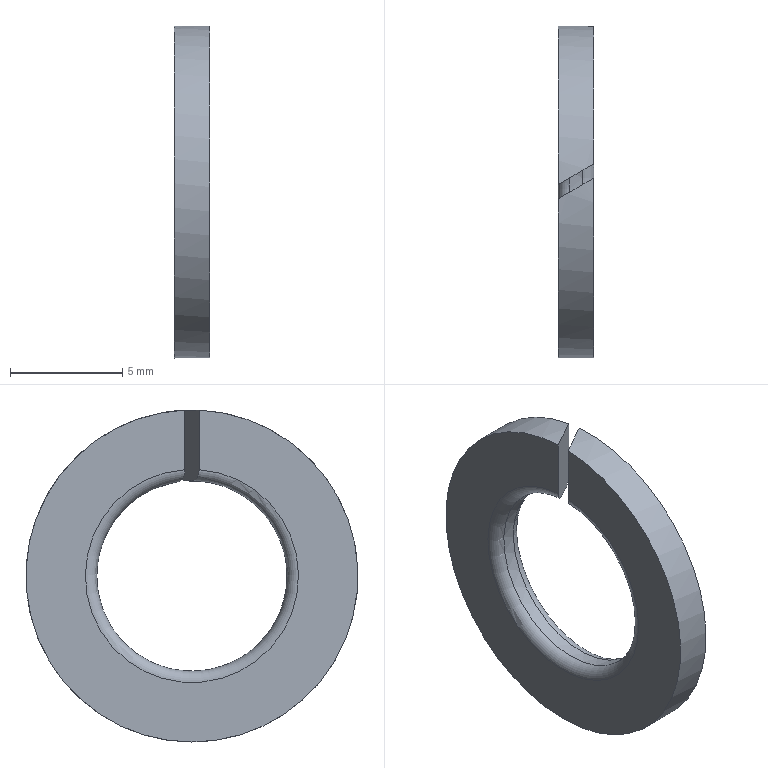Part | STEP file | DIN 128 - A8 | 1 solid | 8 faces | box 1.6 x 14.8 x 14.8 mm | volume 178.348 mm3 | plane 4 | cylinder 2 | torus 2 | commonest cylinder face diameters 8.5 x1 14.8 x1
STEP:
#1=CARTESIAN_POINT('',(0.,0.,0.));
#2=DIRECTION('',(0.,0.,1.));
#3=DIRECTION('',(1.,0.,0.));
#4=AXIS2_PLACEMENT_3D('',#1,#2,#3);
#5=CARTESIAN_POINT('',(1.6,1.244,4.584));
#6=VERTEX_POINT('',#5);
#7=CARTESIAN_POINT('',(1.1,0.9551,4.141));
#8=VERTEX_POINT('',#7);
#9=CARTESIAN_POINT('',(1.6,1.244,4.584));
#10=CARTESIAN_POINT('',(1.6,1.244,4.523));
#11=CARTESIAN_POINT('',(1.587,1.236,4.452));
#12=CARTESIAN_POINT('',(1.542,1.21,4.343));
#13=CARTESIAN_POINT('',(1.503,1.188,4.287));
#14=CARTESIAN_POINT('',(1.419,1.139,4.208));
#15=CARTESIAN_POINT('',(1.358,1.104,4.174));
#16=CARTESIAN_POINT('',(1.242,1.037,4.138));
#17=CARTESIAN_POINT('',(1.164,0.9922,4.133));
#18=CARTESIAN_POINT('',(1.1,0.9551,4.141));
#19=B_SPLINE_CURVE_WITH_KNOTS('',3,(#9,#10,#11,#12,#13,#14,#15,#16,#17,#18),.UNSPECIFIED.,.F.,.F.,(4,2,2,2,4),(0.08409,0.1023,0.1203,0.1398,0.1622),.UNSPECIFIED.);
#20=CARTESIAN_POINT('',(0.,0.32,0.));
#21=DIRECTION('',(-0.5,0.866,0.));
#22=DIRECTION('',(0.,0.,1.));
#23=AXIS2_PLACEMENT_3D('',#20,#21,#22);
#24=PLANE('',#23);
#25=CARTESIAN_POINT('',(4.584,1.848));
#26=CARTESIAN_POINT('',(4.523,1.848));
#27=CARTESIAN_POINT('',(4.452,1.832));
#28=CARTESIAN_POINT('',(4.343,1.78));
#29=CARTESIAN_POINT('',(4.287,1.735));
#30=CARTESIAN_POINT('',(4.208,1.638));
#31=CARTESIAN_POINT('',(4.174,1.568));
#32=CARTESIAN_POINT('',(4.138,1.434));
#33=CARTESIAN_POINT('',(4.133,1.344));
#34=CARTESIAN_POINT('',(4.141,1.27));
#35=B_SPLINE_CURVE_WITH_KNOTS('',3,(#25,#26,#27,#28,#29,#30,#31,#32,#33,#34),.UNSPECIFIED.,.F.,.F.,(4,2,2,2,4),(0.08409,0.1023,0.1203,0.1398,0.1622),.UNSPECIFIED.);
#36=(GEOMETRIC_REPRESENTATION_CONTEXT(2)PARAMETRIC_REPRESENTATION_CONTEXT()REPRESENTATION_CONTEXT('',''));
#37=DEFINITIONAL_REPRESENTATION('',(#35),#36);
#38=PCURVE('',#24,#37);
#39=CARTESIAN_POINT('',(1.1,0.,0.));
#40=DIRECTION('',(-1.,0.,0.));
#41=DIRECTION('',(0.,0.,1.));
#42=AXIS2_PLACEMENT_3D('',#39,#40,#41);
#43=TOROIDAL_SURFACE('',#42,4.75,0.5);
#44=CARTESIAN_POINT('',(0.2649,4.712));
#45=CARTESIAN_POINT('',(0.2656,4.69));
#46=CARTESIAN_POINT('',(0.2668,4.642));
#47=CARTESIAN_POINT('',(0.2684,4.567));
#48=CARTESIAN_POINT('',(0.2698,4.491));
#49=CARTESIAN_POINT('',(0.2708,4.414));
#50=CARTESIAN_POINT('',(0.2713,4.341));
#51=CARTESIAN_POINT('',(0.2714,4.27));
#52=CARTESIAN_POINT('',(0.2711,4.193));
#53=CARTESIAN_POINT('',(0.2704,4.116));
#54=CARTESIAN_POINT('',(0.2693,4.04));
#55=CARTESIAN_POINT('',(0.2679,3.967));
#56=CARTESIAN_POINT('',(0.2661,3.898));
#57=CARTESIAN_POINT('',(0.2638,3.824));
#58=CARTESIAN_POINT('',(0.2611,3.751));
#59=CARTESIAN_POINT('',(0.2581,3.678));
#60=CARTESIAN_POINT('',(0.2549,3.607));
#61=CARTESIAN_POINT('',(0.2516,3.542));
#62=CARTESIAN_POINT('',(0.2479,3.475));
#63=CARTESIAN_POINT('',(0.2439,3.407));
#64=CARTESIAN_POINT('',(0.2397,3.338));
#65=CARTESIAN_POINT('',(0.2354,3.27));
#66=CARTESIAN_POINT('',(0.231,3.204));
#67=CARTESIAN_POINT('',(0.2281,3.162));
#68=CARTESIAN_POINT('',(0.2267,3.142));
#69=B_SPLINE_CURVE_WITH_KNOTS('',3,(#44,#45,#46,#47,#48,#49,#50,#51,#52,#53,#54,#55,#56,#57,#58,#59,#60,#61,#62,#63,#64,#65,#66,#67,#68),.UNSPECIFIED.,.F.,.F.,(4,1,1,1,1,1,1,1,1,1,1,1,1,1,1,1,1,1,1,1,1,1,4),(0.08409,0.08764,0.09119,0.09474,0.09829,0.1018,0.1054,0.1089,0.1125,0.116,0.1196,0.1231,0.1267,0.1302,0.1338,0.1373,0.1409,0.1444,0.148,0.1515,0.1551,0.1586,0.1622),.QUASI_UNIFORM_KNOTS.);
#70=(GEOMETRIC_REPRESENTATION_CONTEXT(2)PARAMETRIC_REPRESENTATION_CONTEXT()REPRESENTATION_CONTEXT('',''));
#71=DEFINITIONAL_REPRESENTATION('',(#69),#70);
#72=PCURVE('',#43,#71);
#73=SURFACE_CURVE('',#19,(#38,#72),.PCURVE_S1.);
#74=EDGE_CURVE('',#6,#8,#73,.T.);
#75=ORIENTED_EDGE('',*,*,#74,.F.);
#76=CARTESIAN_POINT('',(1.6,1.244,7.295));
#77=VERTEX_POINT('',#76);
#78=CARTESIAN_POINT('',(1.6,1.244,0.));
#79=DIRECTION('',(0.,0.,-1.));
#80=VECTOR('',#79,1.);
#81=LINE('',#78,#80);
#82=CARTESIAN_POINT('',(0.,1.848));
#83=DIRECTION('',(-1.,0.));
#84=VECTOR('',#83,1.);
#85=LINE('',#82,#84);
#86=(GEOMETRIC_REPRESENTATION_CONTEXT(2)PARAMETRIC_REPRESENTATION_CONTEXT()REPRESENTATION_CONTEXT('',''));
#87=DEFINITIONAL_REPRESENTATION('',(#85),#86);
#88=PCURVE('',#24,#87);
#89=CARTESIAN_POINT('',(1.6,0.,0.));
#90=DIRECTION('',(-1.,0.,0.));
#91=DIRECTION('',(0.,0.,1.));
#92=AXIS2_PLACEMENT_3D('',#89,#90,#91);
#93=PLANE('',#92);
#94=CARTESIAN_POINT('',(0.,1.244));
#95=DIRECTION('',(-1.,0.));
#96=VECTOR('',#95,1.);
#97=LINE('',#94,#96);
#98=(GEOMETRIC_REPRESENTATION_CONTEXT(2)PARAMETRIC_REPRESENTATION_CONTEXT()REPRESENTATION_CONTEXT('',''));
#99=DEFINITIONAL_REPRESENTATION('',(#97),#98);
#100=PCURVE('',#93,#99);
#101=SURFACE_CURVE('',#81,(#88,#100),.PCURVE_S1.);
#102=EDGE_CURVE('',#77,#6,#101,.T.);
#103=ORIENTED_EDGE('',*,*,#102,.F.);
#104=CARTESIAN_POINT('',(0.,0.32,7.393));
#105=VERTEX_POINT('',#104);
#106=CARTESIAN_POINT('',(-0.5543,0.,0.));
#107=DIRECTION('',(-0.5,0.866,0.));
#108=DIRECTION('',(-0.866,-0.5,0.));
#109=AXIS2_PLACEMENT_3D('',#106,#107,#108);
#110=ELLIPSE('',#109,14.8,7.4);
#111=CARTESIAN_POINT('',(0.,-0.64));
#112=DIRECTION('',(0.,-1.));
#113=AXIS2_PLACEMENT_2D('',#111,#112);
#114=ELLIPSE('',#113,14.8,7.4);
#115=(GEOMETRIC_REPRESENTATION_CONTEXT(2)PARAMETRIC_REPRESENTATION_CONTEXT()REPRESENTATION_CONTEXT('',''));
#116=DEFINITIONAL_REPRESENTATION('',(#114),#115);
#117=PCURVE('',#24,#116);
#118=CARTESIAN_POINT('',(0.,0.,0.));
#119=DIRECTION('',(1.,0.,0.));
#120=DIRECTION('',(0.,-1.,0.));
#121=AXIS2_PLACEMENT_3D('',#118,#119,#120);
#122=CYLINDRICAL_SURFACE('',#121,7.4);
#123=CARTESIAN_POINT('',(4.669,0.));
#124=CARTESIAN_POINT('',(4.544,1.6));
#125=B_SPLINE_CURVE_WITH_KNOTS('',1,(#123,#124),.UNSPECIFIED.,.F.,.F.,(2,2),(1.614,1.74),.PIECEWISE_BEZIER_KNOTS.);
#126=(GEOMETRIC_REPRESENTATION_CONTEXT(2)PARAMETRIC_REPRESENTATION_CONTEXT()REPRESENTATION_CONTEXT('',''));
#127=DEFINITIONAL_REPRESENTATION('',(#125),#126);
#128=PCURVE('',#122,#127);
#129=SURFACE_CURVE('',#110,(#117,#128),.PCURVE_S1.);
#130=EDGE_CURVE('',#105,#77,#129,.T.);
#131=ORIENTED_EDGE('',*,*,#130,.F.);
#132=CARTESIAN_POINT('',(0.,0.32,4.739));
#133=VERTEX_POINT('',#132);
#134=CARTESIAN_POINT('',(0.,0.32,0.));
#135=DIRECTION('',(0.,0.,1.));
#136=VECTOR('',#135,1.);
#137=LINE('',#134,#136);
#138=CARTESIAN_POINT('',(0.,0.));
#139=DIRECTION('',(1.,0.));
#140=VECTOR('',#139,1.);
#141=LINE('',#138,#140);
#142=(GEOMETRIC_REPRESENTATION_CONTEXT(2)PARAMETRIC_REPRESENTATION_CONTEXT()REPRESENTATION_CONTEXT('',''));
#143=DEFINITIONAL_REPRESENTATION('',(#141),#142);
#144=PCURVE('',#24,#143);
#145=CARTESIAN_POINT('',(0.,0.,0.));
#146=DIRECTION('',(-1.,0.,0.));
#147=DIRECTION('',(0.,0.,1.));
#148=AXIS2_PLACEMENT_3D('',#145,#146,#147);
#149=PLANE('',#148);
#150=CARTESIAN_POINT('',(0.,0.32));
#151=DIRECTION('',(1.,0.));
#152=VECTOR('',#151,1.);
#153=LINE('',#150,#152);
#154=(GEOMETRIC_REPRESENTATION_CONTEXT(2)PARAMETRIC_REPRESENTATION_CONTEXT()REPRESENTATION_CONTEXT('',''));
#155=DEFINITIONAL_REPRESENTATION('',(#153),#154);
#156=PCURVE('',#149,#155);
#157=SURFACE_CURVE('',#137,(#144,#156),.PCURVE_S1.);
#158=EDGE_CURVE('',#133,#105,#157,.T.);
#159=ORIENTED_EDGE('',*,*,#158,.F.);
#160=CARTESIAN_POINT('',(0.5,0.6087,4.206));
#161=VERTEX_POINT('',#160);
#162=CARTESIAN_POINT('',(0.5,0.6087,4.206));
#163=CARTESIAN_POINT('',(0.4347,0.571,4.212));
#164=CARTESIAN_POINT('',(0.3585,0.527,4.234));
#165=CARTESIAN_POINT('',(0.2419,0.4596,4.293));
#166=CARTESIAN_POINT('',(0.1797,0.4237,4.34));
#167=CARTESIAN_POINT('',(0.09502,0.3749,4.435));
#168=CARTESIAN_POINT('',(0.05578,0.3522,4.498));
#169=CARTESIAN_POINT('',(0.01303,0.3275,4.612));
#170=CARTESIAN_POINT('',(0.,0.32,4.68));
#171=CARTESIAN_POINT('',(0.,0.32,4.739));
#172=B_SPLINE_CURVE_WITH_KNOTS('',3,(#162,#163,#164,#165,#166,#167,#168,#169,#170,#171),.UNSPECIFIED.,.F.,.F.,(4,2,2,2,4),(0.1609,0.1835,0.205,0.2245,0.2421),.UNSPECIFIED.);
#173=CARTESIAN_POINT('',(4.206,0.5774));
#174=CARTESIAN_POINT('',(4.212,0.502));
#175=CARTESIAN_POINT('',(4.234,0.4139));
#176=CARTESIAN_POINT('',(4.293,0.2793));
#177=CARTESIAN_POINT('',(4.34,0.2075));
#178=CARTESIAN_POINT('',(4.435,0.1097));
#179=CARTESIAN_POINT('',(4.498,0.06441));
#180=CARTESIAN_POINT('',(4.612,0.01505));
#181=CARTESIAN_POINT('',(4.68,0.));
#182=CARTESIAN_POINT('',(4.739,0.));
#183=B_SPLINE_CURVE_WITH_KNOTS('',3,(#173,#174,#175,#176,#177,#178,#179,#180,#181,#182),.UNSPECIFIED.,.F.,.F.,(4,2,2,2,4),(0.1609,0.1835,0.205,0.2245,0.2421),.UNSPECIFIED.);
#184=(GEOMETRIC_REPRESENTATION_CONTEXT(2)PARAMETRIC_REPRESENTATION_CONTEXT()REPRESENTATION_CONTEXT('',''));
#185=DEFINITIONAL_REPRESENTATION('',(#183),#184);
#186=PCURVE('',#24,#185);
#187=CARTESIAN_POINT('',(0.5,0.,0.));
#188=DIRECTION('',(1.,0.,0.));
#189=DIRECTION('',(0.,0.,-1.));
#190=AXIS2_PLACEMENT_3D('',#187,#188,#189);
#191=TOROIDAL_SURFACE('',#190,4.75,0.5);
#192=CARTESIAN_POINT('',(9.281,3.142));
#193=CARTESIAN_POINT('',(9.283,3.163));
#194=CARTESIAN_POINT('',(9.286,3.207));
#195=CARTESIAN_POINT('',(9.29,3.275));
#196=CARTESIAN_POINT('',(9.295,3.344));
#197=CARTESIAN_POINT('',(9.3,3.413));
#198=CARTESIAN_POINT('',(9.305,3.482));
#199=CARTESIAN_POINT('',(9.309,3.547));
#200=CARTESIAN_POINT('',(9.314,3.612));
#201=CARTESIAN_POINT('',(9.318,3.681));
#202=CARTESIAN_POINT('',(9.322,3.752));
#203=CARTESIAN_POINT('',(9.327,3.823));
#204=CARTESIAN_POINT('',(9.331,3.894));
#205=CARTESIAN_POINT('',(9.335,3.962));
#206=CARTESIAN_POINT('',(9.338,4.031));
#207=CARTESIAN_POINT('',(9.341,4.105));
#208=CARTESIAN_POINT('',(9.345,4.18));
#209=CARTESIAN_POINT('',(9.348,4.256));
#210=CARTESIAN_POINT('',(9.35,4.329));
#211=CARTESIAN_POINT('',(9.352,4.401));
#212=CARTESIAN_POINT('',(9.354,4.478));
#213=CARTESIAN_POINT('',(9.356,4.558));
#214=CARTESIAN_POINT('',(9.357,4.637));
#215=CARTESIAN_POINT('',(9.357,4.688));
#216=CARTESIAN_POINT('',(9.357,4.712));
#217=B_SPLINE_CURVE_WITH_KNOTS('',3,(#192,#193,#194,#195,#196,#197,#198,#199,#200,#201,#202,#203,#204,#205,#206,#207,#208,#209,#210,#211,#212,#213,#214,#215,#216),.UNSPECIFIED.,.F.,.F.,(4,1,1,1,1,1,1,1,1,1,1,1,1,1,1,1,1,1,1,1,1,1,4),(0.1609,0.1645,0.1682,0.1719,0.1756,0.1793,0.183,0.1867,0.1904,0.1941,0.1978,0.2015,0.2052,0.2088,0.2125,0.2162,0.2199,0.2236,0.2273,0.231,0.2347,0.2384,0.2421),.QUASI_UNIFORM_KNOTS.);
#218=(GEOMETRIC_REPRESENTATION_CONTEXT(2)PARAMETRIC_REPRESENTATION_CONTEXT()REPRESENTATION_CONTEXT('',''));
#219=DEFINITIONAL_REPRESENTATION('',(#217),#218);
#220=PCURVE('',#191,#219);
#221=SURFACE_CURVE('',#172,(#186,#220),.PCURVE_S1.);
#222=EDGE_CURVE('',#161,#133,#221,.T.);
#223=ORIENTED_EDGE('',*,*,#222,.F.);
#224=CARTESIAN_POINT('',(-0.5543,0.,0.));
#225=DIRECTION('',(0.5,-0.866,0.));
#226=DIRECTION('',(-0.866,-0.5,0.));
#227=AXIS2_PLACEMENT_3D('',#224,#225,#226);
#228=ELLIPSE('',#227,8.5,4.25);
#229=CARTESIAN_POINT('',(0.,-9.14));
#230=CARTESIAN_POINT('',(-7.361,-9.14));
#231=CARTESIAN_POINT('',(-3.681,3.61));
#232=CARTESIAN_POINT('',(0.,16.36));
#233=CARTESIAN_POINT('',(3.681,3.61));
#234=CARTESIAN_POINT('',(7.361,-9.14));
#235=CARTESIAN_POINT('',(0.,-9.14));
#236=(BOUNDED_CURVE()B_SPLINE_CURVE(2,(#229,#230,#231,#232,#233,#234,#235),.UNSPECIFIED.,.T.,.F.)B_SPLINE_CURVE_WITH_KNOTS((1,2,2,2,2,1),(-2.094,0.,2.094,4.189,6.283,8.378),.UNSPECIFIED.)CURVE()GEOMETRIC_REPRESENTATION_ITEM()RATIONAL_B_SPLINE_CURVE((1.,0.5,1.,0.5,1.,0.5,1.))REPRESENTATION_ITEM(''));
#237=(GEOMETRIC_REPRESENTATION_CONTEXT(2)PARAMETRIC_REPRESENTATION_CONTEXT()REPRESENTATION_CONTEXT('',''));
#238=DEFINITIONAL_REPRESENTATION('',(#236),#237);
#239=PCURVE('',#24,#238);
#240=CARTESIAN_POINT('',(0.,0.,0.));
#241=DIRECTION('',(1.,0.,0.));
#242=DIRECTION('',(0.,-1.,0.));
#243=AXIS2_PLACEMENT_3D('',#240,#241,#242);
#244=CYLINDRICAL_SURFACE('',#243,4.25);
#245=CARTESIAN_POINT('',(4.486,1.1));
#246=CARTESIAN_POINT('',(4.569,0.5));
#247=B_SPLINE_CURVE_WITH_KNOTS('',1,(#245,#246),.UNSPECIFIED.,.F.,.F.,(2,2),(4.486,4.569),.PIECEWISE_BEZIER_KNOTS.);
#248=(GEOMETRIC_REPRESENTATION_CONTEXT(2)PARAMETRIC_REPRESENTATION_CONTEXT()REPRESENTATION_CONTEXT('',''));
#249=DEFINITIONAL_REPRESENTATION('',(#247),#248);
#250=PCURVE('',#244,#249);
#251=SURFACE_CURVE('',#228,(#239,#250),.PCURVE_S1.);
#252=EDGE_CURVE('',#8,#161,#251,.T.);
#253=ORIENTED_EDGE('',*,*,#252,.F.);
#254=EDGE_LOOP('',(#75,#103,#131,#159,#223,#253));
#255=FACE_BOUND('',#254,.T.);
#256=ADVANCED_FACE('',(#255),#24,.F.);
#257=CARTESIAN_POINT('',(1.1,0.3151,4.238));
#258=VERTEX_POINT('',#257);
#259=CARTESIAN_POINT('',(1.6,0.6038,4.711));
#260=VERTEX_POINT('',#259);
#261=CARTESIAN_POINT('',(1.1,0.3151,4.238));
#262=CARTESIAN_POINT('',(1.162,0.3511,4.236));
#263=CARTESIAN_POINT('',(1.237,0.394,4.247));
#264=CARTESIAN_POINT('',(1.35,0.4593,4.289));
#265=CARTESIAN_POINT('',(1.41,0.494,4.325));
#266=CARTESIAN_POINT('',(1.497,0.5441,4.406));
#267=CARTESIAN_POINT('',(1.539,0.5683,4.466));
#268=CARTESIAN_POINT('',(1.586,0.5956,4.579));
#269=CARTESIAN_POINT('',(1.6,0.6038,4.65));
#270=CARTESIAN_POINT('',(1.6,0.6038,4.711));
#271=B_SPLINE_CURVE_WITH_KNOTS('',3,(#261,#262,#263,#264,#265,#266,#267,#268,#269,#270),.UNSPECIFIED.,.F.,.F.,(4,2,2,2,4),(0.1598,0.1815,0.201,0.2202,0.2386),.UNSPECIFIED.);
#272=CARTESIAN_POINT('',(1.6,0.6038,0.));
#273=DIRECTION('',(0.5,-0.866,0.));
#274=DIRECTION('',(0.,0.,-1.));
#275=AXIS2_PLACEMENT_3D('',#272,#273,#274);
#276=PLANE('',#275);
#277=CARTESIAN_POINT('',(-4.238,-0.5774));
#278=CARTESIAN_POINT('',(-4.236,-0.5053));
#279=CARTESIAN_POINT('',(-4.247,-0.4195));
#280=CARTESIAN_POINT('',(-4.289,-0.2888));
#281=CARTESIAN_POINT('',(-4.325,-0.2196));
#282=CARTESIAN_POINT('',(-4.406,-0.1194));
#283=CARTESIAN_POINT('',(-4.466,-0.07085));
#284=CARTESIAN_POINT('',(-4.579,-0.01634));
#285=CARTESIAN_POINT('',(-4.65,0.));
#286=CARTESIAN_POINT('',(-4.711,0.));
#287=B_SPLINE_CURVE_WITH_KNOTS('',3,(#277,#278,#279,#280,#281,#282,#283,#284,#285,#286),.UNSPECIFIED.,.F.,.F.,(4,2,2,2,4),(0.1598,0.1815,0.201,0.2202,0.2386),.UNSPECIFIED.);
#288=(GEOMETRIC_REPRESENTATION_CONTEXT(2)PARAMETRIC_REPRESENTATION_CONTEXT()REPRESENTATION_CONTEXT('',''));
#289=DEFINITIONAL_REPRESENTATION('',(#287),#288);
#290=PCURVE('',#276,#289);
#291=CARTESIAN_POINT('',(6.357,3.142));
#292=CARTESIAN_POINT('',(6.359,3.162));
#293=CARTESIAN_POINT('',(6.362,3.205));
#294=CARTESIAN_POINT('',(6.366,3.272));
#295=CARTESIAN_POINT('',(6.371,3.34));
#296=CARTESIAN_POINT('',(6.375,3.409));
#297=CARTESIAN_POINT('',(6.379,3.477));
#298=CARTESIAN_POINT('',(6.383,3.542));
#299=CARTESIAN_POINT('',(6.387,3.607));
#300=CARTESIAN_POINT('',(6.39,3.678));
#301=CARTESIAN_POINT('',(6.394,3.75));
#302=CARTESIAN_POINT('',(6.397,3.822));
#303=CARTESIAN_POINT('',(6.4,3.893));
#304=CARTESIAN_POINT('',(6.403,3.961));
#305=CARTESIAN_POINT('',(6.405,4.034));
#306=CARTESIAN_POINT('',(6.407,4.109));
#307=CARTESIAN_POINT('',(6.409,4.186));
#308=CARTESIAN_POINT('',(6.41,4.262));
#309=CARTESIAN_POINT('',(6.411,4.333));
#310=CARTESIAN_POINT('',(6.412,4.407));
#311=CARTESIAN_POINT('',(6.412,4.485));
#312=CARTESIAN_POINT('',(6.412,4.563));
#313=CARTESIAN_POINT('',(6.411,4.64));
#314=CARTESIAN_POINT('',(6.411,4.689));
#315=CARTESIAN_POINT('',(6.411,4.712));
#316=B_SPLINE_CURVE_WITH_KNOTS('',3,(#291,#292,#293,#294,#295,#296,#297,#298,#299,#300,#301,#302,#303,#304,#305,#306,#307,#308,#309,#310,#311,#312,#313,#314,#315),.UNSPECIFIED.,.F.,.F.,(4,1,1,1,1,1,1,1,1,1,1,1,1,1,1,1,1,1,1,1,1,1,4),(0.1598,0.1634,0.167,0.1706,0.1742,0.1777,0.1813,0.1849,0.1885,0.192,0.1956,0.1992,0.2028,0.2064,0.2099,0.2135,0.2171,0.2207,0.2243,0.2278,0.2314,0.235,0.2386),.QUASI_UNIFORM_KNOTS.);
#317=(GEOMETRIC_REPRESENTATION_CONTEXT(2)PARAMETRIC_REPRESENTATION_CONTEXT()REPRESENTATION_CONTEXT('',''));
#318=DEFINITIONAL_REPRESENTATION('',(#316),#317);
#319=PCURVE('',#43,#318);
#320=SURFACE_CURVE('',#271,(#290,#319),.PCURVE_S1.);
#321=EDGE_CURVE('',#258,#260,#320,.T.);
#322=ORIENTED_EDGE('',*,*,#321,.F.);
#323=CARTESIAN_POINT('',(0.5,-0.03132,4.25));
#324=VERTEX_POINT('',#323);
#325=CARTESIAN_POINT('',(0.5543,0.,0.));
#326=DIRECTION('',(-0.5,0.866,0.));
#327=DIRECTION('',(-0.866,-0.5,0.));
#328=AXIS2_PLACEMENT_3D('',#325,#326,#327);
#329=ELLIPSE('',#328,8.5,4.25);
#330=CARTESIAN_POINT('',(0.,-9.708));
#331=CARTESIAN_POINT('',(-7.361,-9.708));
#332=CARTESIAN_POINT('',(-3.681,3.042));
#333=CARTESIAN_POINT('',(0.,15.792));
#334=CARTESIAN_POINT('',(3.681,3.042));
#335=CARTESIAN_POINT('',(7.361,-9.708));
#336=CARTESIAN_POINT('',(0.,-9.708));
#337=(BOUNDED_CURVE()B_SPLINE_CURVE(2,(#330,#331,#332,#333,#334,#335,#336),.UNSPECIFIED.,.T.,.F.)B_SPLINE_CURVE_WITH_KNOTS((1,2,2,2,2,1),(-2.094,0.,2.094,4.189,6.283,8.378),.UNSPECIFIED.)CURVE()GEOMETRIC_REPRESENTATION_ITEM()RATIONAL_B_SPLINE_CURVE((1.,0.5,1.,0.5,1.,0.5,1.))REPRESENTATION_ITEM(''));
#338=(GEOMETRIC_REPRESENTATION_CONTEXT(2)PARAMETRIC_REPRESENTATION_CONTEXT()REPRESENTATION_CONTEXT('',''));
#339=DEFINITIONAL_REPRESENTATION('',(#337),#338);
#340=PCURVE('',#276,#339);
#341=CARTESIAN_POINT('',(-1.563,0.5));
#342=CARTESIAN_POINT('',(-1.645,1.1));
#343=B_SPLINE_CURVE_WITH_KNOTS('',1,(#341,#342),.UNSPECIFIED.,.F.,.F.,(2,2),(1.563,1.645),.PIECEWISE_BEZIER_KNOTS.);
#344=(GEOMETRIC_REPRESENTATION_CONTEXT(2)PARAMETRIC_REPRESENTATION_CONTEXT()REPRESENTATION_CONTEXT('',''));
#345=DEFINITIONAL_REPRESENTATION('',(#343),#344);
#346=PCURVE('',#244,#345);
#347=SURFACE_CURVE('',#329,(#340,#346),.PCURVE_S1.);
#348=EDGE_CURVE('',#324,#258,#347,.T.);
#349=ORIENTED_EDGE('',*,*,#348,.F.);
#350=CARTESIAN_POINT('',(0.,-0.32,4.739));
#351=VERTEX_POINT('',#350);
#352=CARTESIAN_POINT('',(0.,-0.32,4.739));
#353=CARTESIAN_POINT('',(0.,-0.32,4.681));
#354=CARTESIAN_POINT('',(0.01305,-0.3125,4.612));
#355=CARTESIAN_POINT('',(0.05638,-0.2874,4.502));
#356=CARTESIAN_POINT('',(0.09537,-0.2649,4.443));
#357=CARTESIAN_POINT('',(0.1796,-0.2163,4.355));
#358=CARTESIAN_POINT('',(0.2412,-0.1807,4.314));
#359=CARTESIAN_POINT('',(0.3579,-0.1133,4.265));
#360=CARTESIAN_POINT('',(0.4349,-0.06889,4.25));
#361=CARTESIAN_POINT('',(0.5,-0.03132,4.25));
#362=B_SPLINE_CURVE_WITH_KNOTS('',3,(#352,#353,#354,#355,#356,#357,#358,#359,#360,#361),.UNSPECIFIED.,.F.,.F.,(4,2,2,2,4),(0.08051,0.09807,0.1167,0.1373,0.1598),.UNSPECIFIED.);
#363=CARTESIAN_POINT('',(-4.739,-1.848));
#364=CARTESIAN_POINT('',(-4.681,-1.848));
#365=CARTESIAN_POINT('',(-4.612,-1.832));
#366=CARTESIAN_POINT('',(-4.502,-1.782));
#367=CARTESIAN_POINT('',(-4.443,-1.737));
#368=CARTESIAN_POINT('',(-4.355,-1.64));
#369=CARTESIAN_POINT('',(-4.314,-1.569));
#370=CARTESIAN_POINT('',(-4.265,-1.434));
#371=CARTESIAN_POINT('',(-4.25,-1.345));
#372=CARTESIAN_POINT('',(-4.25,-1.27));
#373=B_SPLINE_CURVE_WITH_KNOTS('',3,(#363,#364,#365,#366,#367,#368,#369,#370,#371,#372),.UNSPECIFIED.,.F.,.F.,(4,2,2,2,4),(0.08051,0.09807,0.1167,0.1373,0.1598),.UNSPECIFIED.);
#374=(GEOMETRIC_REPRESENTATION_CONTEXT(2)PARAMETRIC_REPRESENTATION_CONTEXT()REPRESENTATION_CONTEXT('',''));
#375=DEFINITIONAL_REPRESENTATION('',(#373),#374);
#376=PCURVE('',#276,#375);
#377=CARTESIAN_POINT('',(3.209,4.712));
#378=CARTESIAN_POINT('',(3.209,4.688));
#379=CARTESIAN_POINT('',(3.209,4.639));
#380=CARTESIAN_POINT('',(3.209,4.561));
#381=CARTESIAN_POINT('',(3.209,4.482));
#382=CARTESIAN_POINT('',(3.208,4.404));
#383=CARTESIAN_POINT('',(3.207,4.332));
#384=CARTESIAN_POINT('',(3.206,4.259));
#385=CARTESIAN_POINT('',(3.204,4.183));
#386=CARTESIAN_POINT('',(3.202,4.107));
#387=CARTESIAN_POINT('',(3.199,4.032));
#388=CARTESIAN_POINT('',(3.197,3.961));
#389=CARTESIAN_POINT('',(3.194,3.893));
#390=CARTESIAN_POINT('',(3.19,3.821));
#391=CARTESIAN_POINT('',(3.187,3.749));
#392=CARTESIAN_POINT('',(3.183,3.678));
#393=CARTESIAN_POINT('',(3.179,3.608));
#394=CARTESIAN_POINT('',(3.175,3.544));
#395=CARTESIAN_POINT('',(3.171,3.478));
#396=CARTESIAN_POINT('',(3.167,3.41));
#397=CARTESIAN_POINT('',(3.162,3.341));
#398=CARTESIAN_POINT('',(3.158,3.272));
#399=CARTESIAN_POINT('',(3.153,3.205));
#400=CARTESIAN_POINT('',(3.15,3.162));
#401=CARTESIAN_POINT('',(3.149,3.142));
#402=B_SPLINE_CURVE_WITH_KNOTS('',3,(#377,#378,#379,#380,#381,#382,#383,#384,#385,#386,#387,#388,#389,#390,#391,#392,#393,#394,#395,#396,#397,#398,#399,#400,#401),.UNSPECIFIED.,.F.,.F.,(4,1,1,1,1,1,1,1,1,1,1,1,1,1,1,1,1,1,1,1,1,1,4),(0.08051,0.08411,0.08772,0.09132,0.09493,0.09853,0.1021,0.1057,0.1093,0.113,0.1166,0.1202,0.1238,0.1274,0.131,0.1346,0.1382,0.1418,0.1454,0.149,0.1526,0.1562,0.1598),.QUASI_UNIFORM_KNOTS.);
#403=(GEOMETRIC_REPRESENTATION_CONTEXT(2)PARAMETRIC_REPRESENTATION_CONTEXT()REPRESENTATION_CONTEXT('',''));
#404=DEFINITIONAL_REPRESENTATION('',(#402),#403);
#405=PCURVE('',#191,#404);
#406=SURFACE_CURVE('',#362,(#376,#405),.PCURVE_S1.);
#407=EDGE_CURVE('',#351,#324,#406,.T.);
#408=ORIENTED_EDGE('',*,*,#407,.F.);
#409=CARTESIAN_POINT('',(0.,-0.32,7.393));
#410=VERTEX_POINT('',#409);
#411=CARTESIAN_POINT('',(0.,-0.32,0.));
#412=DIRECTION('',(0.,0.,-1.));
#413=VECTOR('',#412,1.);
#414=LINE('',#411,#413);
#415=CARTESIAN_POINT('',(0.,-1.848));
#416=DIRECTION('',(1.,0.));
#417=VECTOR('',#416,1.);
#418=LINE('',#415,#417);
#419=(GEOMETRIC_REPRESENTATION_CONTEXT(2)PARAMETRIC_REPRESENTATION_CONTEXT()REPRESENTATION_CONTEXT('',''));
#420=DEFINITIONAL_REPRESENTATION('',(#418),#419);
#421=PCURVE('',#276,#420);
#422=CARTESIAN_POINT('',(0.,-0.32));
#423=DIRECTION('',(-1.,0.));
#424=VECTOR('',#423,1.);
#425=LINE('',#422,#424);
#426=(GEOMETRIC_REPRESENTATION_CONTEXT(2)PARAMETRIC_REPRESENTATION_CONTEXT()REPRESENTATION_CONTEXT('',''));
#427=DEFINITIONAL_REPRESENTATION('',(#425),#426);
#428=PCURVE('',#149,#427);
#429=SURFACE_CURVE('',#414,(#421,#428),.PCURVE_S1.);
#430=EDGE_CURVE('',#410,#351,#429,.T.);
#431=ORIENTED_EDGE('',*,*,#430,.F.);
#432=CARTESIAN_POINT('',(1.6,0.6038,7.375));
#433=VERTEX_POINT('',#432);
#434=CARTESIAN_POINT('',(0.5543,0.,0.));
#435=DIRECTION('',(0.5,-0.866,0.));
#436=DIRECTION('',(-0.866,-0.5,0.));
#437=AXIS2_PLACEMENT_3D('',#434,#435,#436);
#438=ELLIPSE('',#437,14.8,7.4);
#439=CARTESIAN_POINT('',(0.,-1.208));
#440=DIRECTION('',(0.,-1.));
#441=AXIS2_PLACEMENT_2D('',#439,#440);
#442=ELLIPSE('',#441,14.8,7.4);
#443=(GEOMETRIC_REPRESENTATION_CONTEXT(2)PARAMETRIC_REPRESENTATION_CONTEXT()REPRESENTATION_CONTEXT('',''));
#444=DEFINITIONAL_REPRESENTATION('',(#442),#443);
#445=PCURVE('',#276,#444);
#446=CARTESIAN_POINT('',(-1.652,1.6));
#447=CARTESIAN_POINT('',(-1.528,0.));
#448=B_SPLINE_CURVE_WITH_KNOTS('',1,(#446,#447),.UNSPECIFIED.,.F.,.F.,(2,2),(4.631,4.756),.PIECEWISE_BEZIER_KNOTS.);
#449=(GEOMETRIC_REPRESENTATION_CONTEXT(2)PARAMETRIC_REPRESENTATION_CONTEXT()REPRESENTATION_CONTEXT('',''));
#450=DEFINITIONAL_REPRESENTATION('',(#448),#449);
#451=PCURVE('',#122,#450);
#452=SURFACE_CURVE('',#438,(#445,#451),.PCURVE_S1.);
#453=EDGE_CURVE('',#433,#410,#452,.T.);
#454=ORIENTED_EDGE('',*,*,#453,.F.);
#455=CARTESIAN_POINT('',(1.6,0.6038,0.));
#456=DIRECTION('',(0.,0.,1.));
#457=VECTOR('',#456,1.);
#458=LINE('',#455,#457);
#459=CARTESIAN_POINT('',(0.,0.));
#460=DIRECTION('',(-1.,0.));
#461=VECTOR('',#460,1.);
#462=LINE('',#459,#461);
#463=(GEOMETRIC_REPRESENTATION_CONTEXT(2)PARAMETRIC_REPRESENTATION_CONTEXT()REPRESENTATION_CONTEXT('',''));
#464=DEFINITIONAL_REPRESENTATION('',(#462),#463);
#465=PCURVE('',#276,#464);
#466=CARTESIAN_POINT('',(0.,0.6038));
#467=DIRECTION('',(1.,0.));
#468=VECTOR('',#467,1.);
#469=LINE('',#466,#468);
#470=(GEOMETRIC_REPRESENTATION_CONTEXT(2)PARAMETRIC_REPRESENTATION_CONTEXT()REPRESENTATION_CONTEXT('',''));
#471=DEFINITIONAL_REPRESENTATION('',(#469),#470);
#472=PCURVE('',#93,#471);
#473=SURFACE_CURVE('',#458,(#465,#472),.PCURVE_S1.);
#474=EDGE_CURVE('',#260,#433,#473,.T.);
#475=ORIENTED_EDGE('',*,*,#474,.F.);
#476=EDGE_LOOP('',(#322,#349,#408,#431,#454,#475));
#477=FACE_BOUND('',#476,.T.);
#478=ADVANCED_FACE('',(#477),#276,.F.);
#479=CARTESIAN_POINT('',(1.1,0.,0.));
#480=DIRECTION('',(-1.,0.,0.));
#481=DIRECTION('',(0.,-1.,0.));
#482=AXIS2_PLACEMENT_3D('',#479,#480,#481);
#483=CIRCLE('',#482,4.25);
#484=CARTESIAN_POINT('',(6.283,1.1));
#485=DIRECTION('',(-1.,0.));
#486=VECTOR('',#485,1.);
#487=LINE('',#484,#486);
#488=(GEOMETRIC_REPRESENTATION_CONTEXT(2)PARAMETRIC_REPRESENTATION_CONTEXT()REPRESENTATION_CONTEXT('',''));
#489=DEFINITIONAL_REPRESENTATION('',(#487),#488);
#490=PCURVE('',#244,#489);
#491=CARTESIAN_POINT('',(-1.571,3.142));
#492=DIRECTION('',(1.,0.));
#493=VECTOR('',#492,1.);
#494=LINE('',#491,#493);
#495=(GEOMETRIC_REPRESENTATION_CONTEXT(2)PARAMETRIC_REPRESENTATION_CONTEXT()REPRESENTATION_CONTEXT('',''));
#496=DEFINITIONAL_REPRESENTATION('',(#494),#495);
#497=PCURVE('',#43,#496);
#498=SURFACE_CURVE('',#483,(#490,#497),.PCURVE_S1.);
#499=EDGE_CURVE('',#8,#258,#498,.T.);
#500=ORIENTED_EDGE('',*,*,#499,.T.);
#501=ORIENTED_EDGE('',*,*,#348,.F.);
#502=CARTESIAN_POINT('',(0.5,0.,0.));
#503=DIRECTION('',(1.,0.,0.));
#504=DIRECTION('',(0.,-1.,0.));
#505=AXIS2_PLACEMENT_3D('',#502,#503,#504);
#506=CIRCLE('',#505,4.25);
#507=CARTESIAN_POINT('',(-6.283,0.5));
#508=DIRECTION('',(1.,0.));
#509=VECTOR('',#508,1.);
#510=LINE('',#507,#509);
#511=(GEOMETRIC_REPRESENTATION_CONTEXT(2)PARAMETRIC_REPRESENTATION_CONTEXT()REPRESENTATION_CONTEXT('',''));
#512=DEFINITIONAL_REPRESENTATION('',(#510),#511);
#513=PCURVE('',#244,#512);
#514=CARTESIAN_POINT('',(-1.571,3.142));
#515=DIRECTION('',(1.,0.));
#516=VECTOR('',#515,1.);
#517=LINE('',#514,#516);
#518=(GEOMETRIC_REPRESENTATION_CONTEXT(2)PARAMETRIC_REPRESENTATION_CONTEXT()REPRESENTATION_CONTEXT('',''));
#519=DEFINITIONAL_REPRESENTATION('',(#517),#518);
#520=PCURVE('',#191,#519);
#521=SURFACE_CURVE('',#506,(#513,#520),.PCURVE_S1.);
#522=EDGE_CURVE('',#324,#161,#521,.T.);
#523=ORIENTED_EDGE('',*,*,#522,.T.);
#524=ORIENTED_EDGE('',*,*,#252,.F.);
#525=EDGE_LOOP('',(#500,#501,#523,#524));
#526=FACE_BOUND('',#525,.F.);
#527=ADVANCED_FACE('',(#526),#244,.F.);
#528=ORIENTED_EDGE('',*,*,#222,.T.);
#529=CARTESIAN_POINT('',(0.,0.,0.));
#530=DIRECTION('',(-1.,0.,0.));
#531=DIRECTION('',(0.,-1.,0.));
#532=AXIS2_PLACEMENT_3D('',#529,#530,#531);
#533=CIRCLE('',#532,4.75);
#534=CARTESIAN_POINT('',(10.996,4.712));
#535=DIRECTION('',(-1.,0.));
#536=VECTOR('',#535,1.);
#537=LINE('',#534,#536);
#538=(GEOMETRIC_REPRESENTATION_CONTEXT(2)PARAMETRIC_REPRESENTATION_CONTEXT()REPRESENTATION_CONTEXT('',''));
#539=DEFINITIONAL_REPRESENTATION('',(#537),#538);
#540=PCURVE('',#191,#539);
#541=CARTESIAN_POINT('',(0.,0.));
#542=DIRECTION('',(0.,-1.));
#543=AXIS2_PLACEMENT_2D('',#541,#542);
#544=CIRCLE('',#543,4.75);
#545=(GEOMETRIC_REPRESENTATION_CONTEXT(2)PARAMETRIC_REPRESENTATION_CONTEXT()REPRESENTATION_CONTEXT('',''));
#546=DEFINITIONAL_REPRESENTATION('',(#544),#545);
#547=PCURVE('',#149,#546);
#548=SURFACE_CURVE('',#533,(#540,#547),.PCURVE_S1.);
#549=EDGE_CURVE('',#133,#351,#548,.T.);
#550=ORIENTED_EDGE('',*,*,#549,.T.);
#551=ORIENTED_EDGE('',*,*,#407,.T.);
#552=ORIENTED_EDGE('',*,*,#522,.T.);
#553=EDGE_LOOP('',(#528,#550,#551,#552));
#554=FACE_BOUND('',#553,.T.);
#555=ADVANCED_FACE('',(#554),#191,.T.);
#556=ORIENTED_EDGE('',*,*,#158,.T.);
#557=CARTESIAN_POINT('',(0.,0.,0.));
#558=DIRECTION('',(-1.,0.,0.));
#559=DIRECTION('',(0.,-1.,0.));
#560=AXIS2_PLACEMENT_3D('',#557,#558,#559);
#561=CIRCLE('',#560,7.4);
#562=CARTESIAN_POINT('',(0.,0.));
#563=DIRECTION('',(0.,-1.));
#564=AXIS2_PLACEMENT_2D('',#562,#563);
#565=CIRCLE('',#564,7.4);
#566=(GEOMETRIC_REPRESENTATION_CONTEXT(2)PARAMETRIC_REPRESENTATION_CONTEXT()REPRESENTATION_CONTEXT('',''));
#567=DEFINITIONAL_REPRESENTATION('',(#565),#566);
#568=PCURVE('',#149,#567);
#569=CARTESIAN_POINT('',(6.283,0.));
#570=DIRECTION('',(-1.,0.));
#571=VECTOR('',#570,1.);
#572=LINE('',#569,#571);
#573=(GEOMETRIC_REPRESENTATION_CONTEXT(2)PARAMETRIC_REPRESENTATION_CONTEXT()REPRESENTATION_CONTEXT('',''));
#574=DEFINITIONAL_REPRESENTATION('',(#572),#573);
#575=PCURVE('',#122,#574);
#576=SURFACE_CURVE('',#561,(#568,#575),.PCURVE_S1.);
#577=EDGE_CURVE('',#105,#410,#576,.T.);
#578=ORIENTED_EDGE('',*,*,#577,.T.);
#579=ORIENTED_EDGE('',*,*,#430,.T.);
#580=ORIENTED_EDGE('',*,*,#549,.F.);
#581=EDGE_LOOP('',(#556,#578,#579,#580));
#582=FACE_BOUND('',#581,.T.);
#583=ADVANCED_FACE('',(#582),#149,.T.);
#584=ORIENTED_EDGE('',*,*,#74,.T.);
#585=ORIENTED_EDGE('',*,*,#499,.T.);
#586=ORIENTED_EDGE('',*,*,#321,.T.);
#587=CARTESIAN_POINT('',(1.6,0.,0.));
#588=DIRECTION('',(1.,0.,0.));
#589=DIRECTION('',(0.,-1.,0.));
#590=AXIS2_PLACEMENT_3D('',#587,#588,#589);
#591=CIRCLE('',#590,4.75);
#592=CARTESIAN_POINT('',(10.996,4.712));
#593=DIRECTION('',(-1.,0.));
#594=VECTOR('',#593,1.);
#595=LINE('',#592,#594);
#596=(GEOMETRIC_REPRESENTATION_CONTEXT(2)PARAMETRIC_REPRESENTATION_CONTEXT()REPRESENTATION_CONTEXT('',''));
#597=DEFINITIONAL_REPRESENTATION('',(#595),#596);
#598=PCURVE('',#43,#597);
#599=CARTESIAN_POINT('',(0.,-4.75));
#600=CARTESIAN_POINT('',(-8.227,-4.75));
#601=CARTESIAN_POINT('',(-4.114,2.375));
#602=CARTESIAN_POINT('',(0.,9.5));
#603=CARTESIAN_POINT('',(4.114,2.375));
#604=CARTESIAN_POINT('',(8.227,-4.75));
#605=CARTESIAN_POINT('',(0.,-4.75));
#606=(BOUNDED_CURVE()B_SPLINE_CURVE(2,(#599,#600,#601,#602,#603,#604,#605),.UNSPECIFIED.,.T.,.F.)B_SPLINE_CURVE_WITH_KNOTS((1,2,2,2,2,1),(-2.094,0.,2.094,4.189,6.283,8.378),.UNSPECIFIED.)CURVE()GEOMETRIC_REPRESENTATION_ITEM()RATIONAL_B_SPLINE_CURVE((1.,0.5,1.,0.5,1.,0.5,1.))REPRESENTATION_ITEM(''));
#607=(GEOMETRIC_REPRESENTATION_CONTEXT(2)PARAMETRIC_REPRESENTATION_CONTEXT()REPRESENTATION_CONTEXT('',''));
#608=DEFINITIONAL_REPRESENTATION('',(#606),#607);
#609=PCURVE('',#93,#608);
#610=SURFACE_CURVE('',#591,(#598,#609),.PCURVE_S1.);
#611=EDGE_CURVE('',#260,#6,#610,.T.);
#612=ORIENTED_EDGE('',*,*,#611,.T.);
#613=EDGE_LOOP('',(#584,#585,#586,#612));
#614=FACE_BOUND('',#613,.T.);
#615=ADVANCED_FACE('',(#614),#43,.T.);
#616=ORIENTED_EDGE('',*,*,#102,.T.);
#617=ORIENTED_EDGE('',*,*,#611,.F.);
#618=ORIENTED_EDGE('',*,*,#474,.T.);
#619=CARTESIAN_POINT('',(1.6,0.,0.));
#620=DIRECTION('',(-1.,0.,0.));
#621=DIRECTION('',(0.,-1.,0.));
#622=AXIS2_PLACEMENT_3D('',#619,#620,#621);
#623=CIRCLE('',#622,7.4);
#624=CARTESIAN_POINT('',(0.,0.));
#625=DIRECTION('',(0.,-1.));
#626=AXIS2_PLACEMENT_2D('',#624,#625);
#627=CIRCLE('',#626,7.4);
#628=(GEOMETRIC_REPRESENTATION_CONTEXT(2)PARAMETRIC_REPRESENTATION_CONTEXT()REPRESENTATION_CONTEXT('',''));
#629=DEFINITIONAL_REPRESENTATION('',(#627),#628);
#630=PCURVE('',#93,#629);
#631=CARTESIAN_POINT('',(6.283,1.6));
#632=DIRECTION('',(-1.,0.));
#633=VECTOR('',#632,1.);
#634=LINE('',#631,#633);
#635=(GEOMETRIC_REPRESENTATION_CONTEXT(2)PARAMETRIC_REPRESENTATION_CONTEXT()REPRESENTATION_CONTEXT('',''));
#636=DEFINITIONAL_REPRESENTATION('',(#634),#635);
#637=PCURVE('',#122,#636);
#638=SURFACE_CURVE('',#623,(#630,#637),.PCURVE_S1.);
#639=EDGE_CURVE('',#77,#433,#638,.T.);
#640=ORIENTED_EDGE('',*,*,#639,.F.);
#641=EDGE_LOOP('',(#616,#617,#618,#640));
#642=FACE_BOUND('',#641,.T.);
#643=ADVANCED_FACE('',(#642),#93,.F.);
#644=ORIENTED_EDGE('',*,*,#130,.T.);
#645=ORIENTED_EDGE('',*,*,#639,.T.);
#646=ORIENTED_EDGE('',*,*,#453,.T.);
#647=ORIENTED_EDGE('',*,*,#577,.F.);
#648=EDGE_LOOP('',(#644,#645,#646,#647));
#649=FACE_BOUND('',#648,.T.);
#650=ADVANCED_FACE('',(#649),#122,.T.);
#651=CLOSED_SHELL('',(#256,#478,#527,#555,#583,#615,#643,#650));
#652=MANIFOLD_SOLID_BREP('',#651);
#653=(LENGTH_UNIT()NAMED_UNIT(*)SI_UNIT(.MILLI.,.METRE.));
#654=UNCERTAINTY_MEASURE_WITH_UNIT(LENGTH_MEASURE(0.001),#653,'','');
#655=(NAMED_UNIT(*)PLANE_ANGLE_UNIT()SI_UNIT($,.RADIAN.));
#656=(NAMED_UNIT(*)SI_UNIT($,.STERADIAN.)SOLID_ANGLE_UNIT());
#657=(GEOMETRIC_REPRESENTATION_CONTEXT(3)GLOBAL_UNCERTAINTY_ASSIGNED_CONTEXT((#654))GLOBAL_UNIT_ASSIGNED_CONTEXT((#653,#655,#656))REPRESENTATION_CONTEXT('',''));
#658=ADVANCED_BREP_SHAPE_REPRESENTATION('',(#4,#652),#657);